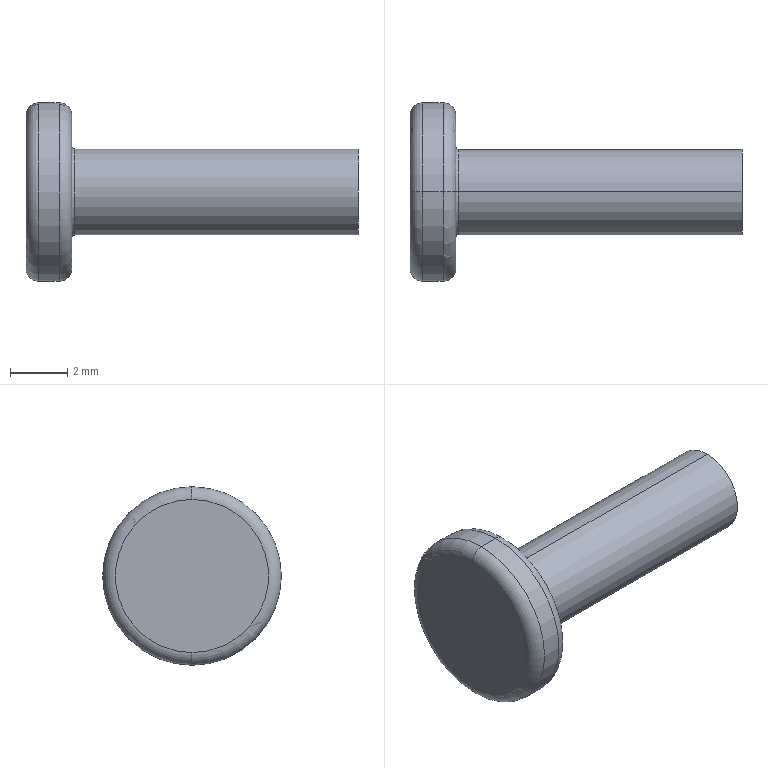Part | SolidWorks | features Revolution 1 | 1 solid | 13 faces | box 11.6 x 6.24 x 6.24 mm | volume 118.025 mm3 | torus 6 | cylinder 4 | plane 3 | commonest cylinder face diameters 3 x2 6.24 x2
STEP:
#1=CARTESIAN_POINT('',(0.4448,0.,3.12));
#2=VERTEX_POINT('',#1);
#3=CARTESIAN_POINT('',(0.4448,0.,-3.12));
#4=VERTEX_POINT('',#3);
#5=CARTESIAN_POINT('',(0.4448,0.,0.));
#6=DIRECTION('',(-1.,0.,0.));
#7=DIRECTION('',(0.,0.,1.));
#8=AXIS2_PLACEMENT_3D('',#5,#6,#7);
#9=CIRCLE('',#8,3.12);
#10=EDGE_CURVE('',#2,#4,#9,.T.);
#11=ORIENTED_EDGE('',*,*,#10,.T.);
#12=CARTESIAN_POINT('',(0.,0.,-2.675));
#13=VERTEX_POINT('',#12);
#14=CARTESIAN_POINT('',(0.4448,0.,-2.675));
#15=DIRECTION('',(0.,1.,0.));
#16=DIRECTION('',(0.,0.,1.));
#17=AXIS2_PLACEMENT_3D('',#14,#15,#16);
#18=CIRCLE('',#17,0.4448);
#19=EDGE_CURVE('',#4,#13,#18,.T.);
#20=ORIENTED_EDGE('',*,*,#19,.T.);
#21=CARTESIAN_POINT('',(0.,0.,2.675));
#22=VERTEX_POINT('',#21);
#23=CARTESIAN_POINT('',(0.,0.,0.));
#24=DIRECTION('',(-1.,0.,0.));
#25=DIRECTION('',(0.,0.,1.));
#26=AXIS2_PLACEMENT_3D('',#23,#24,#25);
#27=CIRCLE('',#26,2.675);
#28=EDGE_CURVE('',#22,#13,#27,.T.);
#29=ORIENTED_EDGE('',*,*,#28,.F.);
#30=CARTESIAN_POINT('',(0.4448,0.,2.675));
#31=DIRECTION('',(0.,-1.,0.));
#32=DIRECTION('',(0.,0.,-1.));
#33=AXIS2_PLACEMENT_3D('',#30,#31,#32);
#34=CIRCLE('',#33,0.4448);
#35=EDGE_CURVE('',#2,#22,#34,.T.);
#36=ORIENTED_EDGE('',*,*,#35,.F.);
#37=EDGE_LOOP('',(#11,#20,#29,#36));
#38=FACE_OUTER_BOUND('',#37,.T.);
#39=CARTESIAN_POINT('',(0.4448,0.,0.));
#40=DIRECTION('',(-1.,0.,0.));
#41=DIRECTION('',(0.,0.,1.));
#42=AXIS2_PLACEMENT_3D('',#39,#40,#41);
#43=TOROIDAL_SURFACE('',#42,2.675,0.4448);
#44=ADVANCED_FACE('',(#38),#43,.T.);
#45=CARTESIAN_POINT('',(1.155,0.,3.12));
#46=VERTEX_POINT('',#45);
#47=CARTESIAN_POINT('',(1.155,0.,-3.12));
#48=VERTEX_POINT('',#47);
#49=CARTESIAN_POINT('',(1.155,0.,0.));
#50=DIRECTION('',(-1.,0.,0.));
#51=DIRECTION('',(0.,0.,1.));
#52=AXIS2_PLACEMENT_3D('',#49,#50,#51);
#53=CIRCLE('',#52,3.12);
#54=EDGE_CURVE('',#46,#48,#53,.T.);
#55=ORIENTED_EDGE('',*,*,#54,.T.);
#56=CARTESIAN_POINT('',(0.,0.,-3.12));
#57=DIRECTION('',(-1.,0.,0.));
#58=VECTOR('',#57,1000.);
#59=LINE('',#56,#58);
#60=EDGE_CURVE('',#48,#4,#59,.T.);
#61=ORIENTED_EDGE('',*,*,#60,.T.);
#62=ORIENTED_EDGE('',*,*,#10,.F.);
#63=CARTESIAN_POINT('',(0.,0.,3.12));
#64=DIRECTION('',(-1.,0.,0.));
#65=VECTOR('',#64,1000.);
#66=LINE('',#63,#65);
#67=EDGE_CURVE('',#46,#2,#66,.T.);
#68=ORIENTED_EDGE('',*,*,#67,.F.);
#69=EDGE_LOOP('',(#55,#61,#62,#68));
#70=FACE_OUTER_BOUND('',#69,.T.);
#71=CARTESIAN_POINT('',(0.,0.,0.));
#72=DIRECTION('',(-1.,0.,0.));
#73=DIRECTION('',(0.,0.,1.));
#74=AXIS2_PLACEMENT_3D('',#71,#72,#73);
#75=CYLINDRICAL_SURFACE('',#74,3.12);
#76=ADVANCED_FACE('',(#70),#75,.T.);
#77=CARTESIAN_POINT('',(1.6,0.,2.675));
#78=VERTEX_POINT('',#77);
#79=CARTESIAN_POINT('',(1.6,0.,-2.675));
#80=VERTEX_POINT('',#79);
#81=CARTESIAN_POINT('',(1.6,0.,0.));
#82=DIRECTION('',(-1.,0.,0.));
#83=DIRECTION('',(0.,0.,1.));
#84=AXIS2_PLACEMENT_3D('',#81,#82,#83);
#85=CIRCLE('',#84,2.675);
#86=EDGE_CURVE('',#78,#80,#85,.T.);
#87=ORIENTED_EDGE('',*,*,#86,.T.);
#88=CARTESIAN_POINT('',(1.155,0.,-2.675));
#89=DIRECTION('',(0.,1.,0.));
#90=DIRECTION('',(0.,0.,1.));
#91=AXIS2_PLACEMENT_3D('',#88,#89,#90);
#92=CIRCLE('',#91,0.4448);
#93=EDGE_CURVE('',#80,#48,#92,.T.);
#94=ORIENTED_EDGE('',*,*,#93,.T.);
#95=ORIENTED_EDGE('',*,*,#54,.F.);
#96=CARTESIAN_POINT('',(1.155,0.,2.675));
#97=DIRECTION('',(0.,-1.,0.));
#98=DIRECTION('',(0.,0.,-1.));
#99=AXIS2_PLACEMENT_3D('',#96,#97,#98);
#100=CIRCLE('',#99,0.4448);
#101=EDGE_CURVE('',#78,#46,#100,.T.);
#102=ORIENTED_EDGE('',*,*,#101,.F.);
#103=EDGE_LOOP('',(#87,#94,#95,#102));
#104=FACE_OUTER_BOUND('',#103,.T.);
#105=CARTESIAN_POINT('',(1.155,0.,0.));
#106=DIRECTION('',(-1.,0.,0.));
#107=DIRECTION('',(0.,0.,1.));
#108=AXIS2_PLACEMENT_3D('',#105,#106,#107);
#109=TOROIDAL_SURFACE('',#108,2.675,0.4448);
#110=ADVANCED_FACE('',(#104),#109,.T.);
#111=CARTESIAN_POINT('',(1.6,0.,-1.6));
#112=VERTEX_POINT('',#111);
#113=CARTESIAN_POINT('',(1.6,0.,1.6));
#114=VERTEX_POINT('',#113);
#115=CARTESIAN_POINT('',(1.6,0.,0.));
#116=DIRECTION('',(-1.,0.,0.));
#117=DIRECTION('',(0.,0.,1.));
#118=AXIS2_PLACEMENT_3D('',#115,#116,#117);
#119=CIRCLE('',#118,1.6);
#120=EDGE_CURVE('',#112,#114,#119,.T.);
#121=ORIENTED_EDGE('',*,*,#120,.F.);
#122=CARTESIAN_POINT('',(1.7,0.,-1.5));
#123=VERTEX_POINT('',#122);
#124=CARTESIAN_POINT('',(1.7,0.,-1.6));
#125=DIRECTION('',(0.,1.,0.));
#126=DIRECTION('',(0.,0.,1.));
#127=AXIS2_PLACEMENT_3D('',#124,#125,#126);
#128=CIRCLE('',#127,0.1);
#129=EDGE_CURVE('',#112,#123,#128,.T.);
#130=ORIENTED_EDGE('',*,*,#129,.T.);
#131=CARTESIAN_POINT('',(1.7,0.,1.5));
#132=VERTEX_POINT('',#131);
#133=CARTESIAN_POINT('',(1.7,0.,0.));
#134=DIRECTION('',(-1.,0.,0.));
#135=DIRECTION('',(0.,0.,1.));
#136=AXIS2_PLACEMENT_3D('',#133,#134,#135);
#137=CIRCLE('',#136,1.5);
#138=EDGE_CURVE('',#123,#132,#137,.T.);
#139=ORIENTED_EDGE('',*,*,#138,.T.);
#140=CARTESIAN_POINT('',(1.7,0.,1.6));
#141=DIRECTION('',(0.,-1.,0.));
#142=DIRECTION('',(0.,0.,-1.));
#143=AXIS2_PLACEMENT_3D('',#140,#141,#142);
#144=CIRCLE('',#143,0.1);
#145=EDGE_CURVE('',#114,#132,#144,.T.);
#146=ORIENTED_EDGE('',*,*,#145,.F.);
#147=EDGE_LOOP('',(#121,#130,#139,#146));
#148=FACE_OUTER_BOUND('',#147,.T.);
#149=CARTESIAN_POINT('',(1.7,0.,0.));
#150=DIRECTION('',(-1.,0.,0.));
#151=DIRECTION('',(0.,0.,1.));
#152=AXIS2_PLACEMENT_3D('',#149,#150,#151);
#153=TOROIDAL_SURFACE('',#152,1.6,0.1);
#154=ADVANCED_FACE('',(#148),#153,.F.);
#155=CARTESIAN_POINT('',(11.6,0.,1.5));
#156=VERTEX_POINT('',#155);
#157=CARTESIAN_POINT('',(11.6,0.,-1.5));
#158=VERTEX_POINT('',#157);
#159=CARTESIAN_POINT('',(11.6,0.,0.));
#160=DIRECTION('',(-1.,0.,0.));
#161=DIRECTION('',(0.,0.,1.));
#162=AXIS2_PLACEMENT_3D('',#159,#160,#161);
#163=CIRCLE('',#162,1.5);
#164=EDGE_CURVE('',#156,#158,#163,.T.);
#165=ORIENTED_EDGE('',*,*,#164,.T.);
#166=CARTESIAN_POINT('',(0.,0.,-1.5));
#167=DIRECTION('',(-1.,0.,0.));
#168=VECTOR('',#167,1000.);
#169=LINE('',#166,#168);
#170=EDGE_CURVE('',#158,#123,#169,.T.);
#171=ORIENTED_EDGE('',*,*,#170,.T.);
#172=CARTESIAN_POINT('',(1.7,0.,0.));
#173=DIRECTION('',(-1.,0.,0.));
#174=DIRECTION('',(0.,0.,1.));
#175=AXIS2_PLACEMENT_3D('',#172,#173,#174);
#176=CIRCLE('',#175,1.5);
#177=EDGE_CURVE('',#132,#123,#176,.T.);
#178=ORIENTED_EDGE('',*,*,#177,.F.);
#179=CARTESIAN_POINT('',(0.,0.,1.5));
#180=DIRECTION('',(-1.,0.,0.));
#181=VECTOR('',#180,1000.);
#182=LINE('',#179,#181);
#183=EDGE_CURVE('',#156,#132,#182,.T.);
#184=ORIENTED_EDGE('',*,*,#183,.F.);
#185=EDGE_LOOP('',(#165,#171,#178,#184));
#186=FACE_OUTER_BOUND('',#185,.T.);
#187=CARTESIAN_POINT('',(0.,0.,0.));
#188=DIRECTION('',(-1.,0.,0.));
#189=DIRECTION('',(0.,0.,1.));
#190=AXIS2_PLACEMENT_3D('',#187,#188,#189);
#191=CYLINDRICAL_SURFACE('',#190,1.5);
#192=ADVANCED_FACE('',(#186),#191,.T.);
#193=ORIENTED_EDGE('',*,*,#164,.F.);
#194=CARTESIAN_POINT('',(11.6,0.,0.));
#195=DIRECTION('',(-1.,0.,0.));
#196=DIRECTION('',(0.,0.,1.));
#197=AXIS2_PLACEMENT_3D('',#194,#195,#196);
#198=CIRCLE('',#197,1.5);
#199=EDGE_CURVE('',#158,#156,#198,.T.);
#200=ORIENTED_EDGE('',*,*,#199,.F.);
#201=EDGE_LOOP('',(#193,#200));
#202=FACE_OUTER_BOUND('',#201,.T.);
#203=CARTESIAN_POINT('',(11.6,1.5,0.));
#204=DIRECTION('',(-1.,0.,0.));
#205=DIRECTION('',(0.,0.,1.));
#206=AXIS2_PLACEMENT_3D('',#203,#204,#205);
#207=PLANE('',#206);
#208=ADVANCED_FACE('',(#202),#207,.F.);
#209=ORIENTED_EDGE('',*,*,#170,.F.);
#210=ORIENTED_EDGE('',*,*,#199,.T.);
#211=ORIENTED_EDGE('',*,*,#183,.T.);
#212=ORIENTED_EDGE('',*,*,#138,.F.);
#213=EDGE_LOOP('',(#209,#210,#211,#212));
#214=FACE_OUTER_BOUND('',#213,.T.);
#215=CARTESIAN_POINT('',(0.,0.,0.));
#216=DIRECTION('',(-1.,0.,0.));
#217=DIRECTION('',(0.,0.,1.));
#218=AXIS2_PLACEMENT_3D('',#215,#216,#217);
#219=CYLINDRICAL_SURFACE('',#218,1.5);
#220=ADVANCED_FACE('',(#214),#219,.T.);
#221=ORIENTED_EDGE('',*,*,#129,.F.);
#222=CARTESIAN_POINT('',(1.6,0.,0.));
#223=DIRECTION('',(-1.,0.,0.));
#224=DIRECTION('',(0.,0.,1.));
#225=AXIS2_PLACEMENT_3D('',#222,#223,#224);
#226=CIRCLE('',#225,1.6);
#227=EDGE_CURVE('',#114,#112,#226,.T.);
#228=ORIENTED_EDGE('',*,*,#227,.F.);
#229=ORIENTED_EDGE('',*,*,#145,.T.);
#230=ORIENTED_EDGE('',*,*,#177,.T.);
#231=EDGE_LOOP('',(#221,#228,#229,#230));
#232=FACE_OUTER_BOUND('',#231,.T.);
#233=CARTESIAN_POINT('',(1.7,0.,0.));
#234=DIRECTION('',(-1.,0.,0.));
#235=DIRECTION('',(0.,0.,1.));
#236=AXIS2_PLACEMENT_3D('',#233,#234,#235);
#237=TOROIDAL_SURFACE('',#236,1.6,0.1);
#238=ADVANCED_FACE('',(#232),#237,.F.);
#239=ORIENTED_EDGE('',*,*,#86,.F.);
#240=CARTESIAN_POINT('',(1.6,0.,0.));
#241=DIRECTION('',(-1.,0.,0.));
#242=DIRECTION('',(0.,0.,1.));
#243=AXIS2_PLACEMENT_3D('',#240,#241,#242);
#244=CIRCLE('',#243,2.675);
#245=EDGE_CURVE('',#80,#78,#244,.T.);
#246=ORIENTED_EDGE('',*,*,#245,.F.);
#247=EDGE_LOOP('',(#239,#246));
#248=FACE_OUTER_BOUND('',#247,.T.);
#249=ORIENTED_EDGE('',*,*,#227,.T.);
#250=ORIENTED_EDGE('',*,*,#120,.T.);
#251=EDGE_LOOP('',(#249,#250));
#252=FACE_BOUND('',#251,.T.);
#253=CARTESIAN_POINT('',(1.6,2.675,0.));
#254=DIRECTION('',(-1.,0.,0.));
#255=DIRECTION('',(0.,0.,1.));
#256=AXIS2_PLACEMENT_3D('',#253,#254,#255);
#257=PLANE('',#256);
#258=ADVANCED_FACE('',(#248,#252),#257,.F.);
#259=ORIENTED_EDGE('',*,*,#93,.F.);
#260=ORIENTED_EDGE('',*,*,#245,.T.);
#261=ORIENTED_EDGE('',*,*,#101,.T.);
#262=CARTESIAN_POINT('',(1.155,0.,0.));
#263=DIRECTION('',(-1.,0.,0.));
#264=DIRECTION('',(0.,0.,1.));
#265=AXIS2_PLACEMENT_3D('',#262,#263,#264);
#266=CIRCLE('',#265,3.12);
#267=EDGE_CURVE('',#48,#46,#266,.T.);
#268=ORIENTED_EDGE('',*,*,#267,.F.);
#269=EDGE_LOOP('',(#259,#260,#261,#268));
#270=FACE_OUTER_BOUND('',#269,.T.);
#271=CARTESIAN_POINT('',(1.155,0.,0.));
#272=DIRECTION('',(-1.,0.,0.));
#273=DIRECTION('',(0.,0.,1.));
#274=AXIS2_PLACEMENT_3D('',#271,#272,#273);
#275=TOROIDAL_SURFACE('',#274,2.675,0.4448);
#276=ADVANCED_FACE('',(#270),#275,.T.);
#277=ORIENTED_EDGE('',*,*,#60,.F.);
#278=ORIENTED_EDGE('',*,*,#267,.T.);
#279=ORIENTED_EDGE('',*,*,#67,.T.);
#280=CARTESIAN_POINT('',(0.4448,0.,0.));
#281=DIRECTION('',(-1.,0.,0.));
#282=DIRECTION('',(0.,0.,1.));
#283=AXIS2_PLACEMENT_3D('',#280,#281,#282);
#284=CIRCLE('',#283,3.12);
#285=EDGE_CURVE('',#4,#2,#284,.T.);
#286=ORIENTED_EDGE('',*,*,#285,.F.);
#287=EDGE_LOOP('',(#277,#278,#279,#286));
#288=FACE_OUTER_BOUND('',#287,.T.);
#289=CARTESIAN_POINT('',(0.,0.,0.));
#290=DIRECTION('',(-1.,0.,0.));
#291=DIRECTION('',(0.,0.,1.));
#292=AXIS2_PLACEMENT_3D('',#289,#290,#291);
#293=CYLINDRICAL_SURFACE('',#292,3.12);
#294=ADVANCED_FACE('',(#288),#293,.T.);
#295=ORIENTED_EDGE('',*,*,#19,.F.);
#296=ORIENTED_EDGE('',*,*,#285,.T.);
#297=ORIENTED_EDGE('',*,*,#35,.T.);
#298=CARTESIAN_POINT('',(0.,0.,0.));
#299=DIRECTION('',(-1.,0.,0.));
#300=DIRECTION('',(0.,0.,1.));
#301=AXIS2_PLACEMENT_3D('',#298,#299,#300);
#302=CIRCLE('',#301,2.675);
#303=EDGE_CURVE('',#13,#22,#302,.T.);
#304=ORIENTED_EDGE('',*,*,#303,.F.);
#305=EDGE_LOOP('',(#295,#296,#297,#304));
#306=FACE_OUTER_BOUND('',#305,.T.);
#307=CARTESIAN_POINT('',(0.4448,0.,0.));
#308=DIRECTION('',(-1.,0.,0.));
#309=DIRECTION('',(0.,0.,1.));
#310=AXIS2_PLACEMENT_3D('',#307,#308,#309);
#311=TOROIDAL_SURFACE('',#310,2.675,0.4448);
#312=ADVANCED_FACE('',(#306),#311,.T.);
#313=ORIENTED_EDGE('',*,*,#28,.T.);
#314=ORIENTED_EDGE('',*,*,#303,.T.);
#315=EDGE_LOOP('',(#313,#314));
#316=FACE_OUTER_BOUND('',#315,.T.);
#317=CARTESIAN_POINT('',(0.,0.,0.));
#318=DIRECTION('',(1.,0.,0.));
#319=DIRECTION('',(0.,0.,-1.));
#320=AXIS2_PLACEMENT_3D('',#317,#318,#319);
#321=PLANE('',#320);
#322=ADVANCED_FACE('',(#316),#321,.F.);
#323=CLOSED_SHELL('',(#44,#76,#110,#154,#192,#208,#220,#238,#258,#276,#294,#312,#322));
#324=MANIFOLD_SOLID_BREP('',#323);
#325=CARTESIAN_POINT('',(0.,0.,0.));
#326=DIRECTION('',(0.,0.,1.));
#327=DIRECTION('',(1.,0.,0.));
#328=AXIS2_PLACEMENT_3D('',#325,#326,#327);
#329=(LENGTH_UNIT()NAMED_UNIT(*)SI_UNIT(.MILLI.,.METRE.));
#330=UNCERTAINTY_MEASURE_WITH_UNIT(LENGTH_MEASURE(0.00001),#329,'','');
#331=(NAMED_UNIT(*)PLANE_ANGLE_UNIT()SI_UNIT($,.RADIAN.));
#332=(NAMED_UNIT(*)SI_UNIT($,.STERADIAN.)SOLID_ANGLE_UNIT());
#333=(GEOMETRIC_REPRESENTATION_CONTEXT(3)GLOBAL_UNCERTAINTY_ASSIGNED_CONTEXT((#330))GLOBAL_UNIT_ASSIGNED_CONTEXT((#329,#331,#332))REPRESENTATION_CONTEXT('',''));
#334=ADVANCED_BREP_SHAPE_REPRESENTATION('',(#324,#328),#333);